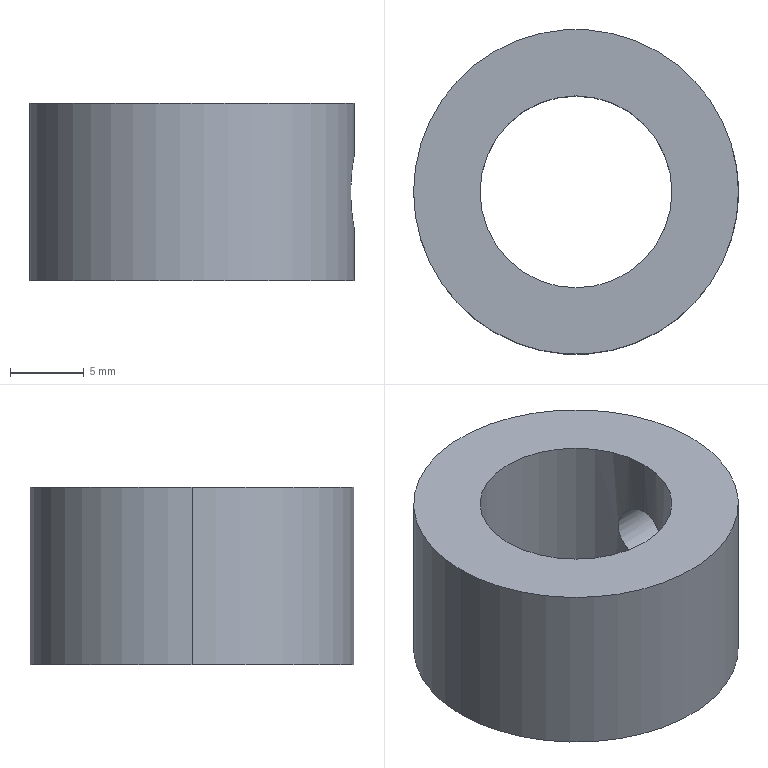Part | SolidWorks | features 3DProfileFeature 1, Extrusion 1, HoleWzd 1 | 1 solid | 10 faces | box 22 x 22 x 12 mm | volume 2905 mm3 | cylinder 6 | cone 2 | plane 2 | commonest cylinder face diameters 4.2 x2 13 x2 22 x2
STEP:
#1=CARTESIAN_POINT('',(6.5,0.,-2.1));
#2=VERTEX_POINT('',#1);
#3=CARTESIAN_POINT('',(6.5,0.,2.1));
#4=VERTEX_POINT('',#3);
#5=CARTESIAN_POINT('',(6.5,0.,-2.1));
#6=CARTESIAN_POINT('',(6.5,-0.1398,-2.1));
#7=CARTESIAN_POINT('',(6.496,-0.277,-2.086));
#8=CARTESIAN_POINT('',(6.478,-0.5467,-2.032));
#9=CARTESIAN_POINT('',(6.466,-0.6806,-1.991));
#10=CARTESIAN_POINT('',(6.434,-0.9346,-1.886));
#11=CARTESIAN_POINT('',(6.415,-1.055,-1.821));
#12=CARTESIAN_POINT('',(6.373,-1.282,-1.669));
#13=CARTESIAN_POINT('',(6.351,-1.389,-1.581));
#14=CARTESIAN_POINT('',(6.283,-1.678,-1.292));
#15=CARTESIAN_POINT('',(6.237,-1.834,-1.059));
#16=CARTESIAN_POINT('',(6.188,-1.991,-0.6808));
#17=CARTESIAN_POINT('',(6.174,-2.032,-0.5475));
#18=CARTESIAN_POINT('',(6.156,-2.086,-0.2759));
#19=CARTESIAN_POINT('',(6.151,-2.1,-0.139));
#20=CARTESIAN_POINT('',(6.151,-2.1,0.137));
#21=CARTESIAN_POINT('',(6.156,-2.086,0.2772));
#22=CARTESIAN_POINT('',(6.174,-2.032,0.5474));
#23=CARTESIAN_POINT('',(6.187,-1.992,0.6788));
#24=CARTESIAN_POINT('',(6.221,-1.886,0.9342));
#25=CARTESIAN_POINT('',(6.24,-1.821,1.055));
#26=CARTESIAN_POINT('',(6.283,-1.669,1.282));
#27=CARTESIAN_POINT('',(6.306,-1.581,1.389));
#28=CARTESIAN_POINT('',(6.351,-1.388,1.582));
#29=CARTESIAN_POINT('',(6.373,-1.283,1.668));
#30=CARTESIAN_POINT('',(6.415,-1.056,1.821));
#31=CARTESIAN_POINT('',(6.434,-0.9327,1.886));
#32=CARTESIAN_POINT('',(6.466,-0.6797,1.992));
#33=CARTESIAN_POINT('',(6.478,-0.5487,2.032));
#34=CARTESIAN_POINT('',(6.496,-0.277,2.086));
#35=CARTESIAN_POINT('',(6.5,-0.1377,2.1));
#36=CARTESIAN_POINT('',(6.5,0.,2.1));
#37=B_SPLINE_CURVE_WITH_KNOTS('',3,(#5,#6,#7,#8,#9,#10,#11,#12,#13,#14,#15,#16,#17,#18,#19,#20,#21,#22,#23,#24,#25,#26,#27,#28,#29,#30,#31,#32,#33,#34,#35,#36),.UNSPECIFIED.,.F.,.F.,(4,2,2,2,2,2,2,2,2,2,2,2,2,2,2,4),(0.,0.0004131,0.0008263,0.001239,0.001653,0.002479,0.002892,0.003305,0.003718,0.004131,0.004545,0.004958,0.005371,0.005784,0.006197,0.00661),.UNSPECIFIED.);
#38=EDGE_CURVE('',#2,#4,#37,.T.);
#39=ORIENTED_EDGE('',*,*,#38,.T.);
#40=CARTESIAN_POINT('',(10.575,0.,2.1));
#41=VERTEX_POINT('',#40);
#42=CARTESIAN_POINT('',(11.,0.,2.1));
#43=DIRECTION('',(1.,0.,0.));
#44=VECTOR('',#43,1000.);
#45=LINE('',#42,#44);
#46=EDGE_CURVE('',#4,#41,#45,.T.);
#47=ORIENTED_EDGE('',*,*,#46,.T.);
#48=CARTESIAN_POINT('',(10.575,0.,-2.1));
#49=VERTEX_POINT('',#48);
#50=CARTESIAN_POINT('',(10.575,0.,0.));
#51=DIRECTION('',(1.,0.,0.));
#52=DIRECTION('',(0.,0.,-1.));
#53=AXIS2_PLACEMENT_3D('',#50,#51,#52);
#54=CIRCLE('',#53,2.1);
#55=EDGE_CURVE('',#41,#49,#54,.T.);
#56=ORIENTED_EDGE('',*,*,#55,.T.);
#57=CARTESIAN_POINT('',(11.,0.,-2.1));
#58=DIRECTION('',(1.,0.,0.));
#59=VECTOR('',#58,1000.);
#60=LINE('',#57,#59);
#61=EDGE_CURVE('',#2,#49,#60,.T.);
#62=ORIENTED_EDGE('',*,*,#61,.F.);
#63=EDGE_LOOP('',(#39,#47,#56,#62));
#64=FACE_OUTER_BOUND('',#63,.T.);
#65=CARTESIAN_POINT('',(11.,0.,0.));
#66=DIRECTION('',(1.,0.,0.));
#67=DIRECTION('',(0.,0.,-1.));
#68=AXIS2_PLACEMENT_3D('',#65,#66,#67);
#69=CYLINDRICAL_SURFACE('',#68,2.1);
#70=ADVANCED_FACE('',(#64),#69,.F.);
#71=ORIENTED_EDGE('',*,*,#55,.F.);
#72=CARTESIAN_POINT('',(11.,0.,2.525));
#73=VERTEX_POINT('',#72);
#74=CARTESIAN_POINT('',(11.,0.,2.525));
#75=DIRECTION('',(0.7071,0.,0.7071));
#76=VECTOR('',#75,1000.);
#77=LINE('',#74,#76);
#78=EDGE_CURVE('',#41,#73,#77,.T.);
#79=ORIENTED_EDGE('',*,*,#78,.T.);
#80=CARTESIAN_POINT('',(11.,0.,-2.525));
#81=VERTEX_POINT('',#80);
#82=CARTESIAN_POINT('',(11.,0.,-2.525));
#83=CARTESIAN_POINT('',(11.,-0.1593,-2.525));
#84=CARTESIAN_POINT('',(10.997,-0.3157,-2.507));
#85=CARTESIAN_POINT('',(10.983,-0.623,-2.435));
#86=CARTESIAN_POINT('',(10.974,-0.7743,-2.381));
#87=CARTESIAN_POINT('',(10.95,-1.057,-2.243));
#88=CARTESIAN_POINT('',(10.936,-1.192,-2.159));
#89=CARTESIAN_POINT('',(10.906,-1.441,-1.964));
#90=CARTESIAN_POINT('',(10.89,-1.555,-1.855));
#91=CARTESIAN_POINT('',(10.859,-1.761,-1.614));
#92=CARTESIAN_POINT('',(10.843,-1.851,-1.485));
#93=CARTESIAN_POINT('',(10.815,-2.008,-1.213));
#94=CARTESIAN_POINT('',(10.803,-2.074,-1.068));
#95=CARTESIAN_POINT('',(10.782,-2.18,-0.7715));
#96=CARTESIAN_POINT('',(10.774,-2.219,-0.6197));
#97=CARTESIAN_POINT('',(10.763,-2.272,-0.309));
#98=CARTESIAN_POINT('',(10.76,-2.285,-0.1495));
#99=CARTESIAN_POINT('',(10.76,-2.285,0.1648));
#100=CARTESIAN_POINT('',(10.763,-2.271,0.3211));
#101=CARTESIAN_POINT('',(10.774,-2.217,0.6318));
#102=CARTESIAN_POINT('',(10.783,-2.175,0.7861));
#103=CARTESIAN_POINT('',(10.804,-2.069,1.081));
#104=CARTESIAN_POINT('',(10.816,-2.003,1.222));
#105=CARTESIAN_POINT('',(10.844,-1.845,1.495));
#106=CARTESIAN_POINT('',(10.86,-1.753,1.624));
#107=CARTESIAN_POINT('',(10.891,-1.549,1.86));
#108=CARTESIAN_POINT('',(10.907,-1.436,1.968));
#109=CARTESIAN_POINT('',(10.936,-1.187,2.162));
#110=CARTESIAN_POINT('',(10.95,-1.053,2.246));
#111=CARTESIAN_POINT('',(10.974,-0.7718,2.382));
#112=CARTESIAN_POINT('',(10.983,-0.6227,2.435));
#113=CARTESIAN_POINT('',(10.997,-0.3135,2.507));
#114=CARTESIAN_POINT('',(11.,-0.1574,2.525));
#115=CARTESIAN_POINT('',(11.,0.,2.525));
#116=B_SPLINE_CURVE_WITH_KNOTS('',3,(#82,#83,#84,#85,#86,#87,#88,#89,#90,#91,#92,#93,#94,#95,#96,#97,#98,#99,#100,#101,#102,#103,#104,#105,#106,#107,#108,#109,#110,#111,#112,#113,#114,#115),.UNSPECIFIED.,.F.,.F.,(4,2,2,2,2,2,2,2,2,2,2,2,2,2,2,2,4),(0.01321,0.01368,0.01415,0.01462,0.0151,0.01557,0.01604,0.01652,0.01699,0.01746,0.01793,0.01841,0.01888,0.01935,0.01983,0.0203,0.02077),.UNSPECIFIED.);
#117=EDGE_CURVE('',#81,#73,#116,.T.);
#118=ORIENTED_EDGE('',*,*,#117,.F.);
#119=CARTESIAN_POINT('',(11.,0.,-2.525));
#120=DIRECTION('',(0.7071,0.,-0.7071));
#121=VECTOR('',#120,1000.);
#122=LINE('',#119,#121);
#123=EDGE_CURVE('',#49,#81,#122,.T.);
#124=ORIENTED_EDGE('',*,*,#123,.F.);
#125=EDGE_LOOP('',(#71,#79,#118,#124));
#126=FACE_OUTER_BOUND('',#125,.T.);
#127=CARTESIAN_POINT('',(11.,0.,0.));
#128=DIRECTION('',(1.,0.,0.));
#129=DIRECTION('',(0.,0.,-1.));
#130=AXIS2_PLACEMENT_3D('',#127,#128,#129);
#131=CONICAL_SURFACE('',#130,2.525,0.7854);
#132=ADVANCED_FACE('',(#126),#131,.F.);
#133=CARTESIAN_POINT('',(-6.5,0.,6.));
#134=VERTEX_POINT('',#133);
#135=CARTESIAN_POINT('',(6.5,0.,6.));
#136=VERTEX_POINT('',#135);
#137=CARTESIAN_POINT('',(0.,0.,6.));
#138=DIRECTION('',(0.,0.,1.));
#139=DIRECTION('',(1.,0.,0.));
#140=AXIS2_PLACEMENT_3D('',#137,#138,#139);
#141=CIRCLE('',#140,6.5);
#142=EDGE_CURVE('',#134,#136,#141,.T.);
#143=ORIENTED_EDGE('',*,*,#142,.T.);
#144=CARTESIAN_POINT('',(6.5,0.,6.));
#145=DIRECTION('',(0.,0.,-1.));
#146=VECTOR('',#145,1000.);
#147=LINE('',#144,#146);
#148=EDGE_CURVE('',#136,#4,#147,.T.);
#149=ORIENTED_EDGE('',*,*,#148,.T.);
#150=ORIENTED_EDGE('',*,*,#38,.F.);
#151=CARTESIAN_POINT('',(6.5,0.,-6.));
#152=VERTEX_POINT('',#151);
#153=CARTESIAN_POINT('',(6.5,0.,6.));
#154=DIRECTION('',(0.,0.,-1.));
#155=VECTOR('',#154,1000.);
#156=LINE('',#153,#155);
#157=EDGE_CURVE('',#2,#152,#156,.T.);
#158=ORIENTED_EDGE('',*,*,#157,.T.);
#159=CARTESIAN_POINT('',(-6.5,0.,-6.));
#160=VERTEX_POINT('',#159);
#161=CARTESIAN_POINT('',(0.,0.,-6.));
#162=DIRECTION('',(0.,0.,1.));
#163=DIRECTION('',(1.,0.,0.));
#164=AXIS2_PLACEMENT_3D('',#161,#162,#163);
#165=CIRCLE('',#164,6.5);
#166=EDGE_CURVE('',#160,#152,#165,.T.);
#167=ORIENTED_EDGE('',*,*,#166,.F.);
#168=CARTESIAN_POINT('',(-6.5,0.,6.));
#169=DIRECTION('',(0.,0.,-1.));
#170=VECTOR('',#169,1000.);
#171=LINE('',#168,#170);
#172=EDGE_CURVE('',#134,#160,#171,.T.);
#173=ORIENTED_EDGE('',*,*,#172,.F.);
#174=EDGE_LOOP('',(#143,#149,#150,#158,#167,#173));
#175=FACE_OUTER_BOUND('',#174,.T.);
#176=CARTESIAN_POINT('',(0.,0.,6.));
#177=DIRECTION('',(0.,0.,-1.));
#178=DIRECTION('',(-1.,0.,0.));
#179=AXIS2_PLACEMENT_3D('',#176,#177,#178);
#180=CYLINDRICAL_SURFACE('',#179,6.5);
#181=ADVANCED_FACE('',(#175),#180,.F.);
#182=CARTESIAN_POINT('',(11.,0.,6.));
#183=VERTEX_POINT('',#182);
#184=CARTESIAN_POINT('',(-11.,0.,6.));
#185=VERTEX_POINT('',#184);
#186=CARTESIAN_POINT('',(0.,0.,6.));
#187=DIRECTION('',(0.,0.,1.));
#188=DIRECTION('',(1.,0.,0.));
#189=AXIS2_PLACEMENT_3D('',#186,#187,#188);
#190=CIRCLE('',#189,11.);
#191=EDGE_CURVE('',#183,#185,#190,.T.);
#192=ORIENTED_EDGE('',*,*,#191,.F.);
#193=CARTESIAN_POINT('',(11.,0.,6.));
#194=DIRECTION('',(0.,0.,-1.));
#195=VECTOR('',#194,1000.);
#196=LINE('',#193,#195);
#197=EDGE_CURVE('',#183,#73,#196,.T.);
#198=ORIENTED_EDGE('',*,*,#197,.T.);
#199=CARTESIAN_POINT('',(11.,0.,2.525));
#200=CARTESIAN_POINT('',(11.,0.1574,2.525));
#201=CARTESIAN_POINT('',(10.996,0.3174,2.506));
#202=CARTESIAN_POINT('',(10.983,0.6237,2.435));
#203=CARTESIAN_POINT('',(10.974,0.7731,2.381));
#204=CARTESIAN_POINT('',(10.95,1.058,2.243));
#205=CARTESIAN_POINT('',(10.936,1.191,2.159));
#206=CARTESIAN_POINT('',(10.906,1.439,1.966));
#207=CARTESIAN_POINT('',(10.89,1.554,1.855));
#208=CARTESIAN_POINT('',(10.844,1.86,1.499));
#209=CARTESIAN_POINT('',(10.814,2.02,1.22));
#210=CARTESIAN_POINT('',(10.782,2.178,0.7763));
#211=CARTESIAN_POINT('',(10.774,2.219,0.6221));
#212=CARTESIAN_POINT('',(10.763,2.272,0.3105));
#213=CARTESIAN_POINT('',(10.76,2.285,0.154));
#214=CARTESIAN_POINT('',(10.76,2.285,-0.1604));
#215=CARTESIAN_POINT('',(10.763,2.271,-0.3199));
#216=CARTESIAN_POINT('',(10.774,2.217,-0.6306));
#217=CARTESIAN_POINT('',(10.783,2.177,-0.782));
#218=CARTESIAN_POINT('',(10.804,2.07,-1.077));
#219=CARTESIAN_POINT('',(10.816,2.003,-1.222));
#220=CARTESIAN_POINT('',(10.844,1.846,-1.494));
#221=CARTESIAN_POINT('',(10.859,1.756,-1.621));
#222=CARTESIAN_POINT('',(10.891,1.551,-1.858));
#223=CARTESIAN_POINT('',(10.907,1.436,-1.969));
#224=CARTESIAN_POINT('',(10.936,1.189,-2.161));
#225=CARTESIAN_POINT('',(10.95,1.056,-2.244));
#226=CARTESIAN_POINT('',(10.974,0.773,-2.381));
#227=CARTESIAN_POINT('',(10.983,0.6219,-2.435));
#228=CARTESIAN_POINT('',(10.997,0.3165,-2.506));
#229=CARTESIAN_POINT('',(11.,0.1592,-2.525));
#230=CARTESIAN_POINT('',(11.,0.,-2.525));
#231=B_SPLINE_CURVE_WITH_KNOTS('',3,(#199,#200,#201,#202,#203,#204,#205,#206,#207,#208,#209,#210,#211,#212,#213,#214,#215,#216,#217,#218,#219,#220,#221,#222,#223,#224,#225,#226,#227,#228,#229,#230),.UNSPECIFIED.,.F.,.F.,(4,2,2,2,2,2,2,2,2,2,2,2,2,2,2,4),(0.005642,0.006115,0.006588,0.00706,0.007533,0.008478,0.008951,0.009424,0.009897,0.01037,0.01084,0.01131,0.01179,0.01226,0.01273,0.01321),.UNSPECIFIED.);
#232=EDGE_CURVE('',#73,#81,#231,.T.);
#233=ORIENTED_EDGE('',*,*,#232,.T.);
#234=CARTESIAN_POINT('',(11.,0.,-6.));
#235=VERTEX_POINT('',#234);
#236=CARTESIAN_POINT('',(11.,0.,6.));
#237=DIRECTION('',(0.,0.,-1.));
#238=VECTOR('',#237,1000.);
#239=LINE('',#236,#238);
#240=EDGE_CURVE('',#81,#235,#239,.T.);
#241=ORIENTED_EDGE('',*,*,#240,.T.);
#242=CARTESIAN_POINT('',(-11.,0.,-6.));
#243=VERTEX_POINT('',#242);
#244=CARTESIAN_POINT('',(0.,0.,-6.));
#245=DIRECTION('',(0.,0.,1.));
#246=DIRECTION('',(1.,0.,0.));
#247=AXIS2_PLACEMENT_3D('',#244,#245,#246);
#248=CIRCLE('',#247,11.);
#249=EDGE_CURVE('',#235,#243,#248,.T.);
#250=ORIENTED_EDGE('',*,*,#249,.T.);
#251=CARTESIAN_POINT('',(-11.,0.,6.));
#252=DIRECTION('',(0.,0.,-1.));
#253=VECTOR('',#252,1000.);
#254=LINE('',#251,#253);
#255=EDGE_CURVE('',#185,#243,#254,.T.);
#256=ORIENTED_EDGE('',*,*,#255,.F.);
#257=EDGE_LOOP('',(#192,#198,#233,#241,#250,#256));
#258=FACE_OUTER_BOUND('',#257,.T.);
#259=CARTESIAN_POINT('',(0.,0.,6.));
#260=DIRECTION('',(0.,0.,-1.));
#261=DIRECTION('',(-1.,0.,0.));
#262=AXIS2_PLACEMENT_3D('',#259,#260,#261);
#263=CYLINDRICAL_SURFACE('',#262,11.);
#264=ADVANCED_FACE('',(#258),#263,.T.);
#265=CARTESIAN_POINT('',(0.,0.,6.));
#266=DIRECTION('',(0.,0.,1.));
#267=DIRECTION('',(1.,0.,0.));
#268=AXIS2_PLACEMENT_3D('',#265,#266,#267);
#269=CIRCLE('',#268,11.);
#270=EDGE_CURVE('',#185,#183,#269,.T.);
#271=ORIENTED_EDGE('',*,*,#270,.T.);
#272=ORIENTED_EDGE('',*,*,#191,.T.);
#273=EDGE_LOOP('',(#271,#272));
#274=FACE_OUTER_BOUND('',#273,.T.);
#275=ORIENTED_EDGE('',*,*,#142,.F.);
#276=CARTESIAN_POINT('',(0.,0.,6.));
#277=DIRECTION('',(0.,0.,1.));
#278=DIRECTION('',(1.,0.,0.));
#279=AXIS2_PLACEMENT_3D('',#276,#277,#278);
#280=CIRCLE('',#279,6.5);
#281=EDGE_CURVE('',#136,#134,#280,.T.);
#282=ORIENTED_EDGE('',*,*,#281,.F.);
#283=EDGE_LOOP('',(#275,#282));
#284=FACE_BOUND('',#283,.T.);
#285=CARTESIAN_POINT('',(0.,0.,6.));
#286=DIRECTION('',(0.,0.,1.));
#287=DIRECTION('',(1.,0.,0.));
#288=AXIS2_PLACEMENT_3D('',#285,#286,#287);
#289=PLANE('',#288);
#290=ADVANCED_FACE('',(#274,#284),#289,.T.);
#291=CARTESIAN_POINT('',(0.,0.,-6.));
#292=DIRECTION('',(0.,0.,1.));
#293=DIRECTION('',(1.,0.,0.));
#294=AXIS2_PLACEMENT_3D('',#291,#292,#293);
#295=CIRCLE('',#294,11.);
#296=EDGE_CURVE('',#243,#235,#295,.T.);
#297=ORIENTED_EDGE('',*,*,#296,.F.);
#298=ORIENTED_EDGE('',*,*,#249,.F.);
#299=EDGE_LOOP('',(#297,#298));
#300=FACE_OUTER_BOUND('',#299,.T.);
#301=ORIENTED_EDGE('',*,*,#166,.T.);
#302=CARTESIAN_POINT('',(0.,0.,-6.));
#303=DIRECTION('',(0.,0.,1.));
#304=DIRECTION('',(1.,0.,0.));
#305=AXIS2_PLACEMENT_3D('',#302,#303,#304);
#306=CIRCLE('',#305,6.5);
#307=EDGE_CURVE('',#152,#160,#306,.T.);
#308=ORIENTED_EDGE('',*,*,#307,.T.);
#309=EDGE_LOOP('',(#301,#308));
#310=FACE_BOUND('',#309,.T.);
#311=CARTESIAN_POINT('',(0.,0.,-6.));
#312=DIRECTION('',(0.,0.,1.));
#313=DIRECTION('',(1.,0.,0.));
#314=AXIS2_PLACEMENT_3D('',#311,#312,#313);
#315=PLANE('',#314);
#316=ADVANCED_FACE('',(#300,#310),#315,.F.);
#317=ORIENTED_EDGE('',*,*,#197,.F.);
#318=ORIENTED_EDGE('',*,*,#270,.F.);
#319=ORIENTED_EDGE('',*,*,#255,.T.);
#320=ORIENTED_EDGE('',*,*,#296,.T.);
#321=ORIENTED_EDGE('',*,*,#240,.F.);
#322=ORIENTED_EDGE('',*,*,#117,.T.);
#323=EDGE_LOOP('',(#317,#318,#319,#320,#321,#322));
#324=FACE_OUTER_BOUND('',#323,.T.);
#325=CARTESIAN_POINT('',(0.,0.,6.));
#326=DIRECTION('',(0.,0.,-1.));
#327=DIRECTION('',(-1.,0.,0.));
#328=AXIS2_PLACEMENT_3D('',#325,#326,#327);
#329=CYLINDRICAL_SURFACE('',#328,11.);
#330=ADVANCED_FACE('',(#324),#329,.T.);
#331=ORIENTED_EDGE('',*,*,#148,.F.);
#332=ORIENTED_EDGE('',*,*,#281,.T.);
#333=ORIENTED_EDGE('',*,*,#172,.T.);
#334=ORIENTED_EDGE('',*,*,#307,.F.);
#335=ORIENTED_EDGE('',*,*,#157,.F.);
#336=CARTESIAN_POINT('',(6.5,0.,2.1));
#337=CARTESIAN_POINT('',(6.5,0.2753,2.1));
#338=CARTESIAN_POINT('',(6.481,0.5533,2.044));
#339=CARTESIAN_POINT('',(6.434,0.9332,1.886));
#340=CARTESIAN_POINT('',(6.415,1.056,1.82));
#341=CARTESIAN_POINT('',(6.373,1.283,1.668));
#342=CARTESIAN_POINT('',(6.351,1.388,1.582));
#343=CARTESIAN_POINT('',(6.283,1.679,1.291));
#344=CARTESIAN_POINT('',(6.237,1.833,1.062));
#345=CARTESIAN_POINT('',(6.187,1.992,0.6788));
#346=CARTESIAN_POINT('',(6.174,2.032,0.5476));
#347=CARTESIAN_POINT('',(6.156,2.086,0.2782));
#348=CARTESIAN_POINT('',(6.151,2.1,0.1383));
#349=CARTESIAN_POINT('',(6.151,2.1,-0.1385));
#350=CARTESIAN_POINT('',(6.156,2.086,-0.2755));
#351=CARTESIAN_POINT('',(6.174,2.032,-0.5466));
#352=CARTESIAN_POINT('',(6.188,1.991,-0.6803));
#353=CARTESIAN_POINT('',(6.237,1.834,-1.06));
#354=CARTESIAN_POINT('',(6.283,1.678,-1.292));
#355=CARTESIAN_POINT('',(6.351,1.389,-1.581));
#356=CARTESIAN_POINT('',(6.373,1.282,-1.669));
#357=CARTESIAN_POINT('',(6.415,1.055,-1.821));
#358=CARTESIAN_POINT('',(6.434,0.9346,-1.886));
#359=CARTESIAN_POINT('',(6.465,0.6809,-1.991));
#360=CARTESIAN_POINT('',(6.478,0.5469,-2.032));
#361=CARTESIAN_POINT('',(6.495,0.2771,-2.086));
#362=CARTESIAN_POINT('',(6.5,0.1397,-2.1));
#363=CARTESIAN_POINT('',(6.5,0.,-2.1));
#364=B_SPLINE_CURVE_WITH_KNOTS('',3,(#336,#337,#338,#339,#340,#341,#342,#343,#344,#345,#346,#347,#348,#349,#350,#351,#352,#353,#354,#355,#356,#357,#358,#359,#360,#361,#362,#363),.UNSPECIFIED.,.F.,.F.,(4,2,2,2,2,2,2,2,2,2,2,2,2,4),(0.00661,0.007436,0.007849,0.008262,0.009088,0.009501,0.009914,0.01033,0.01074,0.01157,0.01198,0.01239,0.01281,0.01322),.UNSPECIFIED.);
#365=EDGE_CURVE('',#4,#2,#364,.T.);
#366=ORIENTED_EDGE('',*,*,#365,.F.);
#367=EDGE_LOOP('',(#331,#332,#333,#334,#335,#366));
#368=FACE_OUTER_BOUND('',#367,.T.);
#369=CARTESIAN_POINT('',(0.,0.,6.));
#370=DIRECTION('',(0.,0.,-1.));
#371=DIRECTION('',(-1.,0.,0.));
#372=AXIS2_PLACEMENT_3D('',#369,#370,#371);
#373=CYLINDRICAL_SURFACE('',#372,6.5);
#374=ADVANCED_FACE('',(#368),#373,.F.);
#375=ORIENTED_EDGE('',*,*,#78,.F.);
#376=CARTESIAN_POINT('',(10.575,0.,0.));
#377=DIRECTION('',(1.,0.,0.));
#378=DIRECTION('',(0.,0.,-1.));
#379=AXIS2_PLACEMENT_3D('',#376,#377,#378);
#380=CIRCLE('',#379,2.1);
#381=EDGE_CURVE('',#49,#41,#380,.T.);
#382=ORIENTED_EDGE('',*,*,#381,.F.);
#383=ORIENTED_EDGE('',*,*,#123,.T.);
#384=ORIENTED_EDGE('',*,*,#232,.F.);
#385=EDGE_LOOP('',(#375,#382,#383,#384));
#386=FACE_OUTER_BOUND('',#385,.T.);
#387=CARTESIAN_POINT('',(11.,0.,0.));
#388=DIRECTION('',(1.,0.,0.));
#389=DIRECTION('',(0.,0.,-1.));
#390=AXIS2_PLACEMENT_3D('',#387,#388,#389);
#391=CONICAL_SURFACE('',#390,2.525,0.7854);
#392=ADVANCED_FACE('',(#386),#391,.F.);
#393=ORIENTED_EDGE('',*,*,#46,.F.);
#394=ORIENTED_EDGE('',*,*,#365,.T.);
#395=ORIENTED_EDGE('',*,*,#61,.T.);
#396=ORIENTED_EDGE('',*,*,#381,.T.);
#397=EDGE_LOOP('',(#393,#394,#395,#396));
#398=FACE_OUTER_BOUND('',#397,.T.);
#399=CARTESIAN_POINT('',(11.,0.,0.));
#400=DIRECTION('',(1.,0.,0.));
#401=DIRECTION('',(0.,0.,-1.));
#402=AXIS2_PLACEMENT_3D('',#399,#400,#401);
#403=CYLINDRICAL_SURFACE('',#402,2.1);
#404=ADVANCED_FACE('',(#398),#403,.F.);
#405=CLOSED_SHELL('',(#70,#132,#181,#264,#290,#316,#330,#374,#392,#404));
#406=MANIFOLD_SOLID_BREP('',#405);
#407=CARTESIAN_POINT('',(0.,0.,0.));
#408=DIRECTION('',(0.,0.,1.));
#409=DIRECTION('',(1.,0.,0.));
#410=AXIS2_PLACEMENT_3D('',#407,#408,#409);
#411=(LENGTH_UNIT()NAMED_UNIT(*)SI_UNIT(.MILLI.,.METRE.));
#412=UNCERTAINTY_MEASURE_WITH_UNIT(LENGTH_MEASURE(0.00001),#411,'','');
#413=(NAMED_UNIT(*)PLANE_ANGLE_UNIT()SI_UNIT($,.RADIAN.));
#414=(NAMED_UNIT(*)SI_UNIT($,.STERADIAN.)SOLID_ANGLE_UNIT());
#415=(GEOMETRIC_REPRESENTATION_CONTEXT(3)GLOBAL_UNCERTAINTY_ASSIGNED_CONTEXT((#412))GLOBAL_UNIT_ASSIGNED_CONTEXT((#411,#413,#414))REPRESENTATION_CONTEXT('',''));
#416=ADVANCED_BREP_SHAPE_REPRESENTATION('',(#406,#410),#415);